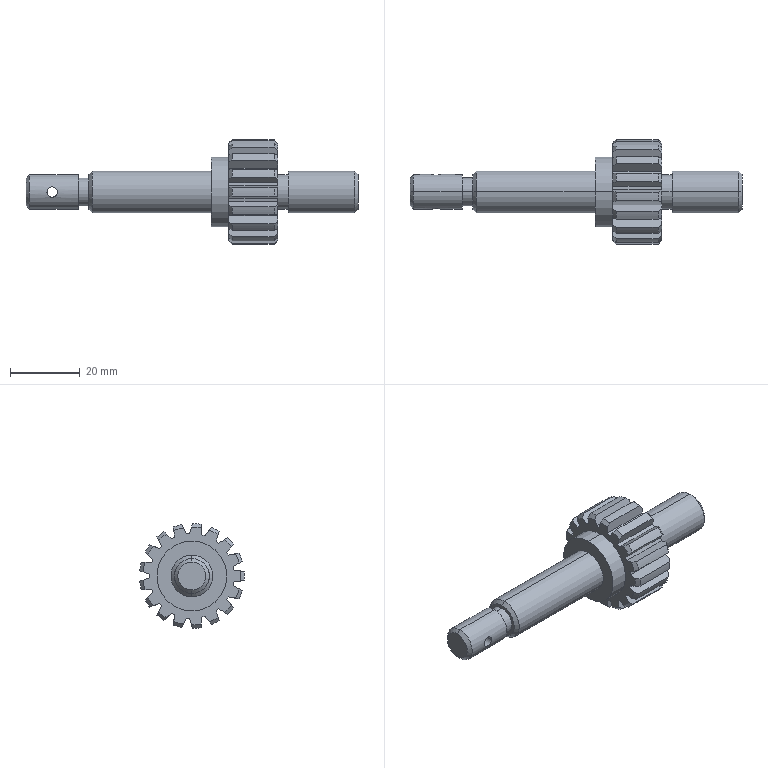Part | SolidWorks | features ICE 7, Chamfer 1, CirPattern 1, Extrusion 1, SweepCut 1 | 1 solid | 132 faces | box 95 x 29.923 x 29.999 mm | volume 17712 mm3 | plane 59 | cone 42 | cylinder 31 | commonest cylinder face diameters 30 x17 10 x4 12 x4 3 x2 8 x2 20 x2